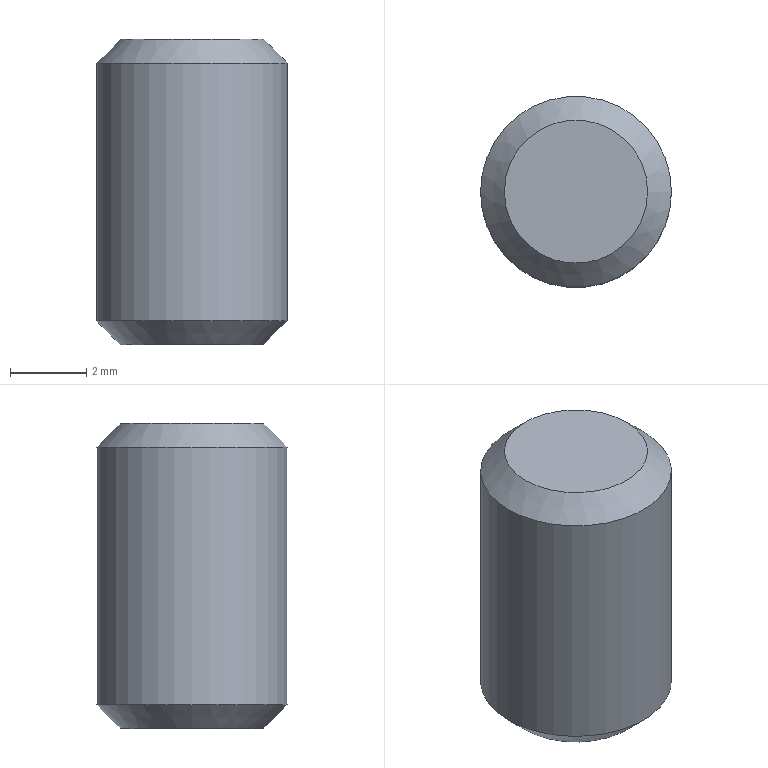Part | NX | features PG_666 2 | 1 solid | 5 faces | box 5 x 5 x 8 mm | volume 151.455 mm3 | plane 2 | cone 2 | cylinder 1 | commonest cylinder face diameters 5 x1
STEP:
#1=CARTESIAN_POINT('',(2393.444,-925.622,943.716));
#2=VERTEX_POINT('',#1);
#3=CARTESIAN_POINT('',(2391.569,-925.622,943.716));
#4=DIRECTION('',(0.,0.,1.));
#5=DIRECTION('',(1.,0.,0.));
#6=AXIS2_PLACEMENT_3D('',#3,#4,#5);
#7=CIRCLE('',#6,1.875);
#8=EDGE_CURVE('',#2,#2,#7,.T.);
#9=ORIENTED_EDGE('',*,*,#8,.T.);
#10=EDGE_LOOP('',(#9));
#11=FACE_BOUND('',#10,.T.);
#12=CARTESIAN_POINT('',(2391.569,-925.622,943.716));
#13=DIRECTION('',(0.,0.,1.));
#14=DIRECTION('',(1.,0.,0.));
#15=AXIS2_PLACEMENT_3D('',#12,#13,#14);
#16=PLANE('',#15);
#17=ADVANCED_FACE('',(#11),#16,.T.);
#18=CARTESIAN_POINT('',(2389.694,-925.622,935.716));
#19=VERTEX_POINT('',#18);
#20=CARTESIAN_POINT('',(2391.569,-925.622,935.716));
#21=DIRECTION('',(0.,0.,-1.));
#22=DIRECTION('',(-1.,0.,0.));
#23=AXIS2_PLACEMENT_3D('',#20,#21,#22);
#24=CIRCLE('',#23,1.875);
#25=EDGE_CURVE('',#19,#19,#24,.T.);
#26=ORIENTED_EDGE('',*,*,#25,.T.);
#27=EDGE_LOOP('',(#26));
#28=FACE_BOUND('',#27,.T.);
#29=CARTESIAN_POINT('',(2391.569,-925.622,935.716));
#30=DIRECTION('',(0.,0.,-1.));
#31=DIRECTION('',(-1.,0.,0.));
#32=AXIS2_PLACEMENT_3D('',#29,#30,#31);
#33=PLANE('',#32);
#34=ADVANCED_FACE('',(#28),#33,.T.);
#35=CARTESIAN_POINT('',(2389.069,-925.622,936.341));
#36=VERTEX_POINT('',#35);
#37=CARTESIAN_POINT('',(2391.569,-925.622,936.341));
#38=DIRECTION('',(0.,0.,-1.));
#39=DIRECTION('',(-1.,0.,0.));
#40=AXIS2_PLACEMENT_3D('',#37,#38,#39);
#41=CIRCLE('',#40,2.5);
#42=EDGE_CURVE('',#36,#36,#41,.F.);
#43=ORIENTED_EDGE('',*,*,#42,.T.);
#44=EDGE_LOOP('',(#43));
#45=FACE_BOUND('',#44,.T.);
#46=CARTESIAN_POINT('',(2394.069,-925.622,943.091));
#47=VERTEX_POINT('',#46);
#48=CARTESIAN_POINT('',(2391.569,-925.622,943.091));
#49=DIRECTION('',(0.,0.,1.));
#50=DIRECTION('',(1.,0.,0.));
#51=AXIS2_PLACEMENT_3D('',#48,#49,#50);
#52=CIRCLE('',#51,2.5);
#53=EDGE_CURVE('',#47,#47,#52,.F.);
#54=ORIENTED_EDGE('',*,*,#53,.T.);
#55=EDGE_LOOP('',(#54));
#56=FACE_BOUND('',#55,.T.);
#57=CARTESIAN_POINT('',(2391.569,-925.622,874.716));
#58=DIRECTION('',(0.,0.,1.));
#59=DIRECTION('',(1.,0.,0.));
#60=AXIS2_PLACEMENT_3D('',#57,#58,#59);
#61=CYLINDRICAL_SURFACE('',#60,2.5);
#62=ADVANCED_FACE('',(#45,#56),#61,.T.);
#63=ORIENTED_EDGE('',*,*,#25,.F.);
#64=EDGE_LOOP('',(#63));
#65=FACE_BOUND('',#64,.T.);
#66=ORIENTED_EDGE('',*,*,#42,.F.);
#67=EDGE_LOOP('',(#66));
#68=FACE_BOUND('',#67,.T.);
#69=CARTESIAN_POINT('',(2391.569,-925.622,936.341));
#70=DIRECTION('',(0.,0.,1.));
#71=DIRECTION('',(1.,0.,0.));
#72=AXIS2_PLACEMENT_3D('',#69,#70,#71);
#73=CONICAL_SURFACE('',#72,2.5,0.7854);
#74=ADVANCED_FACE('',(#65,#68),#73,.T.);
#75=ORIENTED_EDGE('',*,*,#8,.F.);
#76=EDGE_LOOP('',(#75));
#77=FACE_BOUND('',#76,.T.);
#78=ORIENTED_EDGE('',*,*,#53,.F.);
#79=EDGE_LOOP('',(#78));
#80=FACE_BOUND('',#79,.T.);
#81=CARTESIAN_POINT('',(2391.569,-925.622,943.091));
#82=DIRECTION('',(0.,0.,-1.));
#83=DIRECTION('',(-1.,0.,0.));
#84=AXIS2_PLACEMENT_3D('',#81,#82,#83);
#85=CONICAL_SURFACE('',#84,2.5,0.7854);
#86=ADVANCED_FACE('',(#77,#80),#85,.T.);
#87=CLOSED_SHELL('',(#17,#34,#62,#74,#86));
#88=MANIFOLD_SOLID_BREP('',#87);
#89=(LENGTH_UNIT()NAMED_UNIT(*)SI_UNIT(.MILLI.,.METRE.));
#90=UNCERTAINTY_MEASURE_WITH_UNIT(LENGTH_MEASURE(0.00001),#89,'','');
#91=(NAMED_UNIT(*)PLANE_ANGLE_UNIT()SI_UNIT($,.RADIAN.));
#92=(NAMED_UNIT(*)SI_UNIT($,.STERADIAN.)SOLID_ANGLE_UNIT());
#93=(GEOMETRIC_REPRESENTATION_CONTEXT(3)GLOBAL_UNCERTAINTY_ASSIGNED_CONTEXT((#90))GLOBAL_UNIT_ASSIGNED_CONTEXT((#89,#91,#92))REPRESENTATION_CONTEXT('',''));
#94=ADVANCED_BREP_SHAPE_REPRESENTATION('',(#88),#93);